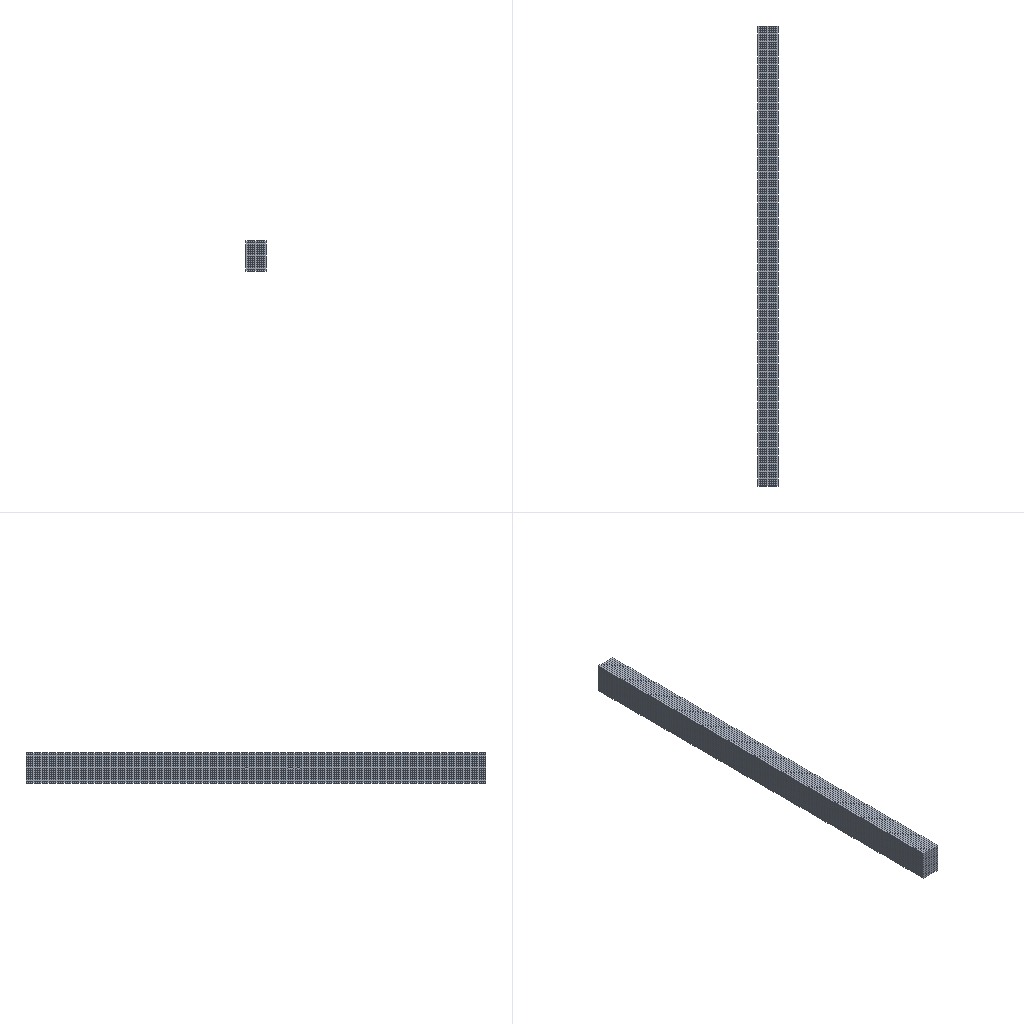Simulation study | ansys workbench
Ansys APDL input file, long lists of numbers shortened:
/batch
/config,noeldb,1     ! force off writing results to database
*get,_wallstrt,active,,time,wall
! ANSYS input file written by Workbench version 2022 R1
! File used for geometry attach: F:\ansys（分析文件汇总)\简支梁有限元分析\零件2.STEP
/title,111--____ (B5)
! ****** Begin Custom Load Command Snippet ******
/COM, ACT Extensions:
/COM,     LSDYNA, 2021.1
/COM,
! ****** End   Custom Load Command Snippet ******
*DIM,_wb_ProjectScratch_dir,string,248
_wb_ProjectScratch_dir(1) = 'F:\ansys（分析文件汇总)\简支梁有限元分析\_ProjectScratch\ScrAA69\'
*DIM,_wb_SolverFiles_dir,string,248
_wb_SolverFiles_dir(1) = 'F:\ansys（分析文件汇总)\简支梁有限元分析\111_files\dp0\SYS\MECH\'
*DIM,_wb_userfiles_dir,string,248
_wb_userfiles_dir(1) = 'F:\ansys（分析文件汇总)\简支梁有限元分析\111_files\user_files\'
/com,--- Data in consistent NMM units. See Solving Units in the help system for more information.
/units,MPA
/nopr
/wb,file,start              !  signify a WB generated input file
/prep7
! Turn off shape checking because checks already performed inside WB mesher.
! See help system for more information.
SHPP,OFF,,NOWARN
/nolist
etcon,set             ! allow ANSYS to choose best KEYOP's for 180x elements, resets any applicable keyopt to MAPDL defaults
/com,*********** Nodes for the whole assembly ***********
nblock,3,,31342
(1i9,3e20.9e3)
        1     4.400000000E+01     2.975000000E+03     7.425000000E+01
! (28492 more lines like these left out)
-1
/wb,elem,start            !  set before creation of elements
/com,*********** Elements for Body 1 "__2-FreeParts|__-__1" ***********
et,1,186
keyo,1,2,1          ! set full integration on SOLID186
eblock,19,solid,,5760
(19i9)
        1        1        1        1        0        0        0        0       20        0        1        1     7540     6809     6678     4998     7575     6808     6683
! (11519 more lines like these left out)
-1
/wb,elem,end               !  done creating elements
/com,*********** Send User Defined Coordinate System(s) ***********
csys,0
toffst,273.15,  ! Temperature offset from absolute zero
/com,*********** Set Reference Temperature ***********
tref,22.
/wb,mat,start              !  starting to send materials
/com,*********** Send Materials ***********
Temperature = 'TEMP' ! Temperature
MP,DENS,1,7.85e-09,	! tonne mm^-3
MP,ALPX,1,1.2e-05,	! C^-1
MP,C,1,434000000,	! mm^2 s^-2 C^-1
MP,KXX,1,60.5,	! tonne mm s^-3 C^-1
MP,RSVX,1,0.00017,	! ohm mm
MP,EX,1,200000,	! tonne s^-2 mm^-1
MP,NUXY,1,0.3,
MP,MURX,1,10000,
/wb,mat,end                !  done sending materials
!************************* Model Summary ********************
!__2-FreeParts|__-__1,	结构钢,	matid,	1
!************************* End Model Summary ********************
! get the diagonal of the bounding box. Needed later for other things
*get,_xmin,node,,mnloc,x
*get,_ymin,node,,mnloc,y
*get,_zmin,node,,mnloc,z
*get,_xmax,node,,mxloc,x
*get,_ymax,node,,mxloc,y
*get,_zmax,node,,mxloc,z
_ASMDIAG=(_xmax-_xmin)*(_xmax-_xmin)+(_ymax-_ymin)*(_ymax-_ymin)+(_zmax-_zmin)*(_zmax-_zmin)
_ASMDIAG=SQRT(_ASMDIAG)
/wb,contact,start          !  starting to send contact
/wb,contact,end            !  done creating contacts
/golist
/wb,load,start             !  starting to send loads
/com,*********** Fixed Supports ***********
CMBLOCK,_FIXEDSU,NODE,       13
(8i10)
      5846      7528      7529      7530      7531      7532      7533     25197
     28330     28332     28334     28336     28338
cmsel,s,_FIXEDSU
d,all,all
nsel,all
/com,******* Constant Zero Displacement X *******
CMBLOCK,_DISPZEROUX,NODE,       13
(8i10)
      5966      7534      7535      7536      7537      7538      7539     25436
     28341     28343     28345     28347     28349
cmsel,s,_DISPZEROUX
d,all,ux,0
nsel,all
/com,******* Constant Zero Displacement Z *******
CMBLOCK,_DISPZEROUZ,NODE,       13
(8i10)
      5966      7534      7535      7536      7537      7538      7539     25436
     28341     28343     28345     28347     28349
cmsel,s,_DISPZEROUZ
d,all,uz,0
nsel,all
/com,*********** Define Force Using Surface Effect Elements ***********
local,12,0,0.,0.,0.,0.,0.,0.
csys,0
et,2,154
eblock,10,,,720
(15i9)
     9217        2        2        2       12     6801     6088     6803     6802    25680    25681    26993    26992
! (719 more lines like these left out)
-1
esel,s,type,,2
keyop,2,2,1                ! Apply load in local coordinate system
keyop,2,7,1                ! Use original area so load is constant in large deformation
esel,all
/gst,on,on
fini
*get,_numnode,node,0,count
*get,_numelem,elem,0,count
*get, _MAXELEMNUM, elem, 0, NUM, MAX
*get, _MAXNODENUM, node, 0, NUM, MAX
*get, _MAXELEMTYPE, etyp, 0, NUM, MAX
*get, _MAXREALCONST, real, 0, NUM, MAX
/go
/wb,load,end               !  done creating loads
/com,--- Number of total nodes = %_numnode%
/com,--- Number of contact elements = 720
/com,--- Number of spring elements = 0
/com,--- Number of bearing elements = 0
/com,--- Number of solid elements = 5760
/com,--- Number of condensed parts = 0
/com,--- Number of total elements = %_numelem%
*get,_wallbsol,active,,time,wall
/com,****************************************************************************
/com,*************************    SOLUTION       ********************************
/com,****************************************************************************
/solu
antype,0                   ! static analysis
_thickRatio=  1     ! Ratio of thick parts in the model
eqsl,pcg,1e-8,,,,,,1
cntr,print,1               ! print out contact info and also make no initial contact an error
dmpoption,emat,no             ! Don't combine emat file for DANSYS
dmpoption,esav,no             ! Don't combine esav file for DANSYS
nldiag,cont,iter           ! print out contact info each equilibrium iteration
rescontrol,,none                 ! Do not keep any restart files
/com,****************************************************
/com,******************* SOLVE FOR LS 1 OF 1 ****************
esel,s,type,,2
nsle
sfe,all,1,pres,1,-8.76122959309761e-018
sfe,all,2,pres,1,0.
sfe,all,3,pres,1,-8.33333333333399e-002
nsel,all
esel,all
/nopr
/gopr
nsub,1,1,1
time,1.
outres,erase
outres,all,none
outres,nsol,all,
outres,rsol,all
outres,eangl,all
outres,etmp,all
outres,veng,all
outres,strs,all,
outres,epel,all,
outres,eppl,all,
outres,cont,all,
! *********** WB SOLVE COMMAND ***********
! check interactive state
*get,ANSINTER_,active,,int
*if,ANSINTER_,ne,0,then
/eof
*endif
solve
/com *************** Write FE CONNECTORS *********
CEWRITE,file,ce,,INTE
/com,****************************************************
/com,*************** FINISHED SOLVE FOR LS 1 *************
*get,_wallasol,active,,time,wall
/nopr
*get,_numnode,node,0,count
*get,_numelem,elem,0,count
*get, _MAXELEMNUM, elem, 0, NUM, MAX
*get, _MAXNODENUM, node, 0, NUM, MAX,,,INTERNAL
*get, _MAXELEMTYPE, etyp, 0, NUM, MAX
*get, _MAXREALCONST, real, 0, NUM, MAX
/gopr
*get,_PCGITER,active,,solu,cgiter
/post1
xmlo,ENCODING,ISO-8859-1
xmlo,parm
/xml,parm,xml
fini
/gopr
*get,_walldone,active,,time,wall
_preptime=(_wallbsol-_wallstrt)*3600
_solvtime=(_wallasol-_wallbsol)*3600
_posttime=(_walldone-_wallasol)*3600
_totaltim=(_walldone-_wallstrt)*3600
*get,_dlbratio,active,0,solu,dlbr
*get,_combtime,active,0,solu,comb
*get,_ssmode,active,0,solu,ssmm
*get,_ndofs,active,0,solu,ndof
*get,_sol_end_time,active,0,set,time
*if,_sol_end_time,eq,1.,then
/fclean				!clean distributed files
*endif
/com,--- Total number of nodes = %_numnode%
/com,--- Total number of elements = %_numelem%
/com,--- Element load balance ratio = %_dlbratio%
/com,--- Time to combine distributed files = %_combtime%
/com,--- Sparse memory mode = %_ssmode%
/com,--- Number of DOF = %_ndofs%
/wb,file,end               ! done with WB generated input